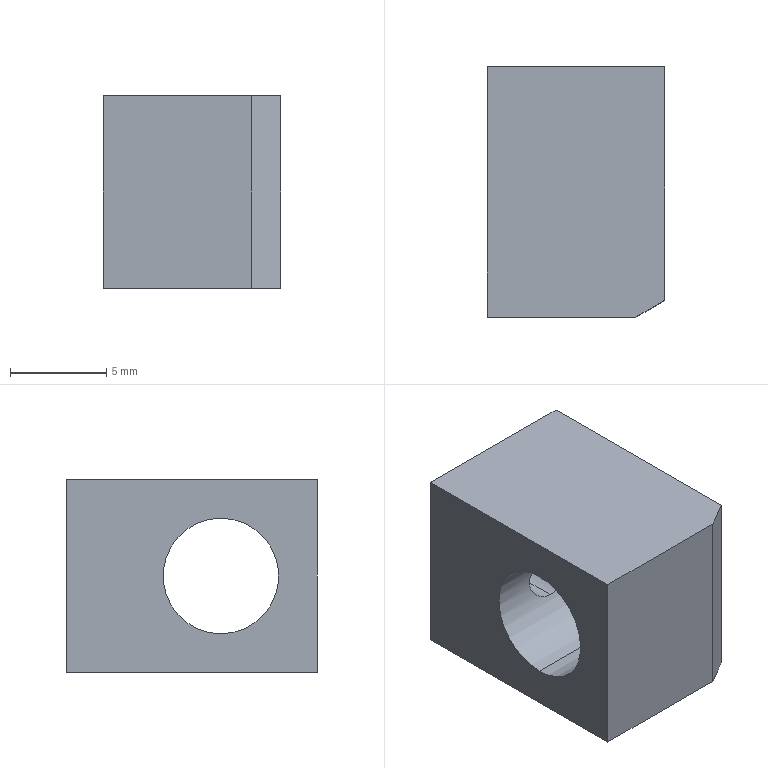Part | STEP file | 22DDSceondwrwet_Default | 1 solid | 18 faces | box 9.2 x 13 x 10 mm | volume 888.519 mm3 | cylinder 8 | plane 8 | cone 2 | commonest cylinder face diameters 2 x2 2.5 x2 6 x2 6.6 x2